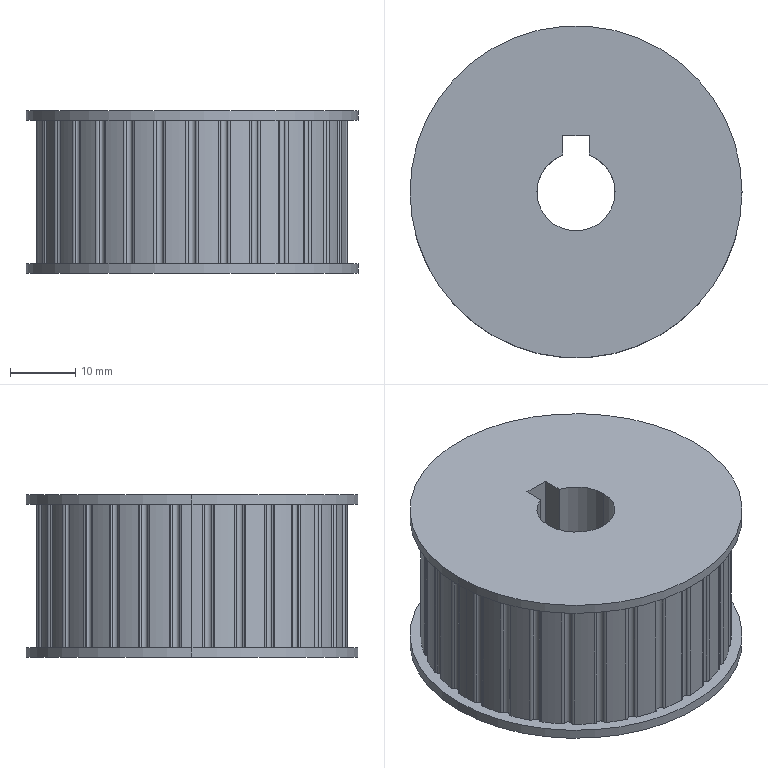Part | 1 solid | 155 faces | box 51 x 51 x 25 mm | volume 42057 mm3 | cylinder 148 | plane 7 | commonest cylinder face diameters 0.96 x70 1.14 x40 47.75 x31 51 x4 12 x3